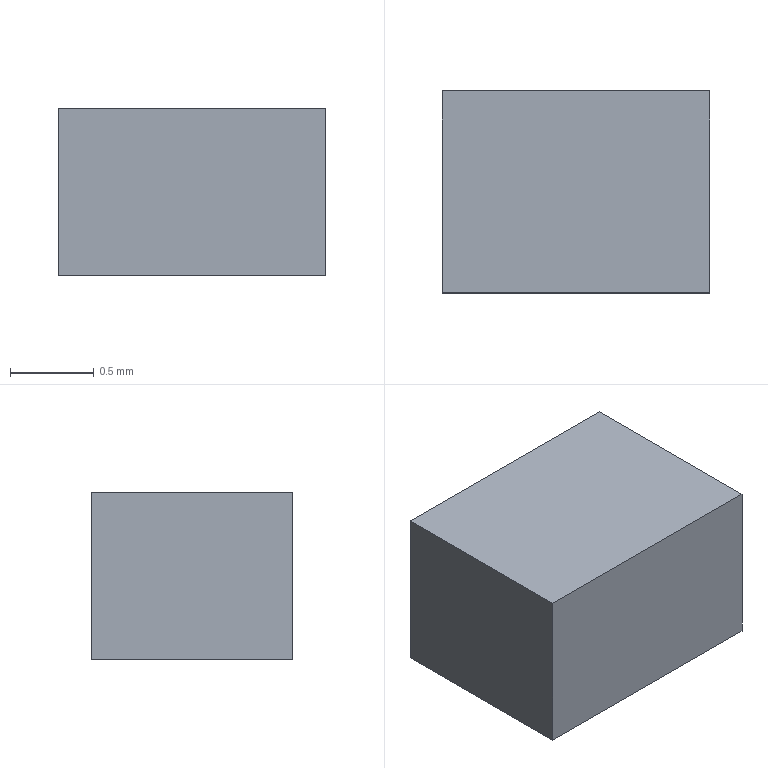Part | Creo | 1 solid | 6 faces | box 1.602 x 1.209 x 1.003 mm | volume 1.943 mm3 | plane 6
STEP:
#1=CARTESIAN_POINT('',(0.,0.,0.));
#2=DIRECTION('',(0.,0.,1.));
#3=DIRECTION('',(1.,0.,0.));
#4=AXIS2_PLACEMENT_3D('',#1,#2,#3);
#5=CARTESIAN_POINT('',(-0.8266,-0.6342,0.));
#6=VERTEX_POINT('',#5);
#7=CARTESIAN_POINT('',(0.775,-0.6342,0.));
#8=VERTEX_POINT('',#7);
#9=CARTESIAN_POINT('',(-0.8266,-0.6342,0.));
#10=DIRECTION('',(1.,0.,0.));
#11=VECTOR('',#10,1.602);
#12=LINE('',#9,#11);
#13=EDGE_CURVE('',#6,#8,#12,.T.);
#14=ORIENTED_EDGE('',*,*,#13,.T.);
#15=CARTESIAN_POINT('',(0.775,0.575,0.));
#16=VERTEX_POINT('',#15);
#17=CARTESIAN_POINT('',(0.775,-0.6342,0.));
#18=DIRECTION('',(0.,1.,0.));
#19=VECTOR('',#18,1.209);
#20=LINE('',#17,#19);
#21=EDGE_CURVE('',#8,#16,#20,.T.);
#22=ORIENTED_EDGE('',*,*,#21,.T.);
#23=CARTESIAN_POINT('',(-0.8266,0.575,0.));
#24=VERTEX_POINT('',#23);
#25=CARTESIAN_POINT('',(0.775,0.575,0.));
#26=DIRECTION('',(-1.,0.,0.));
#27=VECTOR('',#26,1.602);
#28=LINE('',#25,#27);
#29=EDGE_CURVE('',#16,#24,#28,.T.);
#30=ORIENTED_EDGE('',*,*,#29,.T.);
#31=CARTESIAN_POINT('',(-0.8266,0.575,0.));
#32=DIRECTION('',(0.,-1.,0.));
#33=VECTOR('',#32,1.209);
#34=LINE('',#31,#33);
#35=EDGE_CURVE('',#24,#6,#34,.T.);
#36=ORIENTED_EDGE('',*,*,#35,.T.);
#37=EDGE_LOOP('',(#14,#22,#30,#36));
#38=FACE_OUTER_BOUND('',#37,.F.);
#39=CARTESIAN_POINT('',(0.,0.,0.));
#40=DIRECTION('',(0.,0.,1.));
#41=DIRECTION('',(1.,0.,0.));
#42=AXIS2_PLACEMENT_3D('',#39,#40,#41);
#43=PLANE('',#42);
#44=ADVANCED_FACE('',(#38),#43,.F.);
#45=ORIENTED_EDGE('',*,*,#13,.F.);
#46=CARTESIAN_POINT('',(-0.8266,-0.6342,1.003));
#47=VERTEX_POINT('',#46);
#48=CARTESIAN_POINT('',(-0.8266,-0.6342,0.));
#49=DIRECTION('',(0.,0.,1.));
#50=VECTOR('',#49,1.003);
#51=LINE('',#48,#50);
#52=EDGE_CURVE('',#6,#47,#51,.T.);
#53=ORIENTED_EDGE('',*,*,#52,.T.);
#54=CARTESIAN_POINT('',(0.775,-0.6342,1.003));
#55=VERTEX_POINT('',#54);
#56=CARTESIAN_POINT('',(-0.8266,-0.6342,1.003));
#57=DIRECTION('',(1.,0.,0.));
#58=VECTOR('',#57,1.602);
#59=LINE('',#56,#58);
#60=EDGE_CURVE('',#47,#55,#59,.T.);
#61=ORIENTED_EDGE('',*,*,#60,.T.);
#62=CARTESIAN_POINT('',(0.775,-0.6342,0.));
#63=DIRECTION('',(0.,0.,1.));
#64=VECTOR('',#63,1.003);
#65=LINE('',#62,#64);
#66=EDGE_CURVE('',#8,#55,#65,.T.);
#67=ORIENTED_EDGE('',*,*,#66,.F.);
#68=EDGE_LOOP('',(#45,#53,#61,#67));
#69=FACE_OUTER_BOUND('',#68,.F.);
#70=CARTESIAN_POINT('',(-0.8266,-0.6342,0.));
#71=DIRECTION('',(0.,-1.,0.));
#72=DIRECTION('',(1.,0.,0.));
#73=AXIS2_PLACEMENT_3D('',#70,#71,#72);
#74=PLANE('',#73);
#75=ADVANCED_FACE('',(#69),#74,.T.);
#76=ORIENTED_EDGE('',*,*,#35,.F.);
#77=CARTESIAN_POINT('',(-0.8266,0.575,1.003));
#78=VERTEX_POINT('',#77);
#79=CARTESIAN_POINT('',(-0.8266,0.575,0.));
#80=DIRECTION('',(0.,0.,1.));
#81=VECTOR('',#80,1.003);
#82=LINE('',#79,#81);
#83=EDGE_CURVE('',#24,#78,#82,.T.);
#84=ORIENTED_EDGE('',*,*,#83,.T.);
#85=CARTESIAN_POINT('',(-0.8266,0.575,1.003));
#86=DIRECTION('',(0.,-1.,0.));
#87=VECTOR('',#86,1.209);
#88=LINE('',#85,#87);
#89=EDGE_CURVE('',#78,#47,#88,.T.);
#90=ORIENTED_EDGE('',*,*,#89,.T.);
#91=ORIENTED_EDGE('',*,*,#52,.F.);
#92=EDGE_LOOP('',(#76,#84,#90,#91));
#93=FACE_OUTER_BOUND('',#92,.F.);
#94=CARTESIAN_POINT('',(-0.8266,0.575,0.));
#95=DIRECTION('',(-1.,0.,0.));
#96=DIRECTION('',(0.,-1.,0.));
#97=AXIS2_PLACEMENT_3D('',#94,#95,#96);
#98=PLANE('',#97);
#99=ADVANCED_FACE('',(#93),#98,.T.);
#100=ORIENTED_EDGE('',*,*,#29,.F.);
#101=CARTESIAN_POINT('',(0.775,0.575,1.003));
#102=VERTEX_POINT('',#101);
#103=CARTESIAN_POINT('',(0.775,0.575,0.));
#104=DIRECTION('',(0.,0.,1.));
#105=VECTOR('',#104,1.003);
#106=LINE('',#103,#105);
#107=EDGE_CURVE('',#16,#102,#106,.T.);
#108=ORIENTED_EDGE('',*,*,#107,.T.);
#109=CARTESIAN_POINT('',(0.775,0.575,1.003));
#110=DIRECTION('',(-1.,0.,0.));
#111=VECTOR('',#110,1.602);
#112=LINE('',#109,#111);
#113=EDGE_CURVE('',#102,#78,#112,.T.);
#114=ORIENTED_EDGE('',*,*,#113,.T.);
#115=ORIENTED_EDGE('',*,*,#83,.F.);
#116=EDGE_LOOP('',(#100,#108,#114,#115));
#117=FACE_OUTER_BOUND('',#116,.F.);
#118=CARTESIAN_POINT('',(0.775,0.575,0.));
#119=DIRECTION('',(0.,1.,0.));
#120=DIRECTION('',(-1.,0.,0.));
#121=AXIS2_PLACEMENT_3D('',#118,#119,#120);
#122=PLANE('',#121);
#123=ADVANCED_FACE('',(#117),#122,.T.);
#124=ORIENTED_EDGE('',*,*,#21,.F.);
#125=ORIENTED_EDGE('',*,*,#66,.T.);
#126=CARTESIAN_POINT('',(0.775,-0.6342,1.003));
#127=DIRECTION('',(0.,1.,0.));
#128=VECTOR('',#127,1.209);
#129=LINE('',#126,#128);
#130=EDGE_CURVE('',#55,#102,#129,.T.);
#131=ORIENTED_EDGE('',*,*,#130,.T.);
#132=ORIENTED_EDGE('',*,*,#107,.F.);
#133=EDGE_LOOP('',(#124,#125,#131,#132));
#134=FACE_OUTER_BOUND('',#133,.F.);
#135=CARTESIAN_POINT('',(0.775,-0.6342,0.));
#136=DIRECTION('',(1.,0.,0.));
#137=DIRECTION('',(0.,1.,0.));
#138=AXIS2_PLACEMENT_3D('',#135,#136,#137);
#139=PLANE('',#138);
#140=ADVANCED_FACE('',(#134),#139,.T.);
#141=ORIENTED_EDGE('',*,*,#60,.F.);
#142=ORIENTED_EDGE('',*,*,#89,.F.);
#143=ORIENTED_EDGE('',*,*,#113,.F.);
#144=ORIENTED_EDGE('',*,*,#130,.F.);
#145=EDGE_LOOP('',(#141,#142,#143,#144));
#146=FACE_OUTER_BOUND('',#145,.F.);
#147=CARTESIAN_POINT('',(0.,0.,1.003));
#148=DIRECTION('',(0.,0.,1.));
#149=DIRECTION('',(1.,0.,0.));
#150=AXIS2_PLACEMENT_3D('',#147,#148,#149);
#151=PLANE('',#150);
#152=ADVANCED_FACE('',(#146),#151,.T.);
#153=CLOSED_SHELL('',(#44,#75,#99,#123,#140,#152));
#154=MANIFOLD_SOLID_BREP('',#153);
#155=(LENGTH_UNIT()NAMED_UNIT(*)SI_UNIT(.MILLI.,.METRE.));
#156=UNCERTAINTY_MEASURE_WITH_UNIT(LENGTH_MEASURE(0.0002244),#155,'','');
#157=(NAMED_UNIT(*)PLANE_ANGLE_UNIT()SI_UNIT($,.RADIAN.));
#158=PLANE_ANGLE_MEASURE_WITH_UNIT(PLANE_ANGLE_MEASURE(0.01745),#157);
#159=(CONVERSION_BASED_UNIT('DEGREE',#158)NAMED_UNIT(*)PLANE_ANGLE_UNIT());
#160=(NAMED_UNIT(*)SI_UNIT($,.STERADIAN.)SOLID_ANGLE_UNIT());
#161=(GEOMETRIC_REPRESENTATION_CONTEXT(3)GLOBAL_UNCERTAINTY_ASSIGNED_CONTEXT((#156))GLOBAL_UNIT_ASSIGNED_CONTEXT((#155,#159,#160))REPRESENTATION_CONTEXT('',''));
#162=ADVANCED_BREP_SHAPE_REPRESENTATION('',(#4,#154),#161);